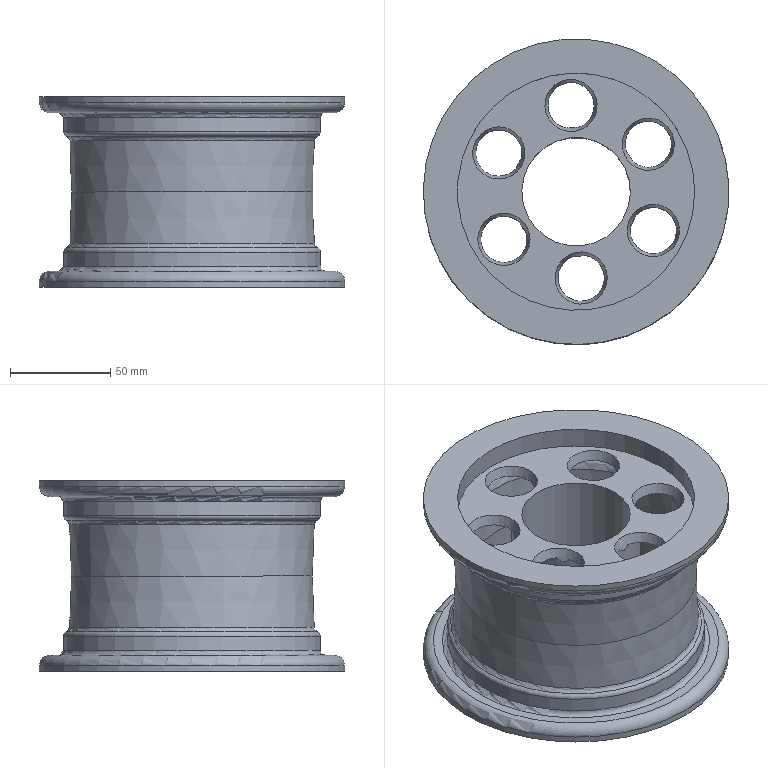Part | NX | features solid 2 | 1 solid | 44 faces | box 152.002 x 152.003 x 95.006 mm | volume 380615 mm3 | cone 16 | cylinder 10 | torus 10 | plane 8 | commonest cylinder face diameters 118 x4 128 x2 152 x2 54 x1 64 x1
STEP:
#1=CARTESIAN_POINT('',(-519.305,-904.645,30.012));
#2=VERTEX_POINT('',#1);
#3=CARTESIAN_POINT('',(-484.115,-958.102,30.014));
#4=DIRECTION('',(0.0000242,-0.00003327,-1.));
#5=DIRECTION('',(-0.5498,0.8353,-0.00004109));
#6=AXIS2_PLACEMENT_3D('',#3,#4,#5);
#7=CIRCLE('',#6,64.);
#8=EDGE_CURVE('',#2,#2,#7,.T.);
#9=ORIENTED_EDGE('',*,*,#8,.F.);
#10=EDGE_LOOP('',(#9));
#11=FACE_BOUND('',#10,.T.);
#12=CARTESIAN_POINT('',(-519.305,-904.644,37.012));
#13=VERTEX_POINT('',#12);
#14=CARTESIAN_POINT('',(-484.115,-958.102,37.014));
#15=DIRECTION('',(0.0000242,-0.00003327,-1.));
#16=DIRECTION('',(-0.5498,0.8353,-0.00004109));
#17=AXIS2_PLACEMENT_3D('',#14,#15,#16);
#18=CIRCLE('',#17,64.);
#19=EDGE_CURVE('',#13,#13,#18,.T.);
#20=ORIENTED_EDGE('',*,*,#19,.T.);
#21=EDGE_LOOP('',(#20));
#22=FACE_BOUND('',#21,.T.);
#23=CARTESIAN_POINT('',(-484.116,-958.1,73.347));
#24=DIRECTION('',(0.0000242,-0.00003327,-1.));
#25=DIRECTION('',(-0.5498,0.8353,-0.00004109));
#26=AXIS2_PLACEMENT_3D('',#23,#24,#25);
#27=CYLINDRICAL_SURFACE('',#26,64.);
#28=ADVANCED_FACE('',(#11,#22),#27,.T.);
#29=CARTESIAN_POINT('',(-518.46,-905.929,27.704));
#30=VERTEX_POINT('',#29);
#31=CARTESIAN_POINT('',(-484.115,-958.102,27.707));
#32=DIRECTION('',(0.0000242,-0.00003327,-1.));
#33=DIRECTION('',(-0.5498,0.8353,-0.00004109));
#34=AXIS2_PLACEMENT_3D('',#31,#32,#33);
#35=CIRCLE('',#34,62.462);
#36=EDGE_CURVE('',#30,#30,#35,.T.);
#37=ORIENTED_EDGE('',*,*,#36,.F.);
#38=EDGE_LOOP('',(#37));
#39=FACE_BOUND('',#38,.T.);
#40=ORIENTED_EDGE('',*,*,#8,.T.);
#41=EDGE_LOOP('',(#40));
#42=FACE_BOUND('',#41,.T.);
#43=CARTESIAN_POINT('',(-484.115,-958.102,30.014));
#44=DIRECTION('',(0.0000242,-0.00003327,-1.));
#45=DIRECTION('',(-0.5498,0.8353,-0.00004109));
#46=AXIS2_PLACEMENT_3D('',#43,#44,#45);
#47=TOROIDAL_SURFACE('',#46,61.5,2.5);
#48=ADVANCED_FACE('',(#39,#42),#47,.T.);
#49=CARTESIAN_POINT('',(-517.615,-907.212,25.488));
#50=VERTEX_POINT('',#49);
#51=CARTESIAN_POINT('',(-484.115,-958.102,25.49));
#52=DIRECTION('',(0.0000242,-0.00003327,-1.));
#53=DIRECTION('',(-0.5498,0.8353,-0.00004109));
#54=AXIS2_PLACEMENT_3D('',#51,#52,#53);
#55=CIRCLE('',#54,60.926);
#56=EDGE_CURVE('',#50,#50,#55,.T.);
#57=ORIENTED_EDGE('',*,*,#56,.F.);
#58=EDGE_LOOP('',(#57));
#59=FACE_BOUND('',#58,.T.);
#60=ORIENTED_EDGE('',*,*,#36,.T.);
#61=EDGE_LOOP('',(#60));
#62=FACE_BOUND('',#61,.T.);
#63=CARTESIAN_POINT('',(-484.115,-958.102,25.399));
#64=DIRECTION('',(0.0000242,-0.00003327,-1.));
#65=DIRECTION('',(-0.5498,0.8353,-0.00004109));
#66=AXIS2_PLACEMENT_3D('',#63,#64,#65);
#67=TOROIDAL_SURFACE('',#66,63.425,2.5);
#68=ADVANCED_FACE('',(#59,#62),#67,.F.);
#69=CARTESIAN_POINT('',(-517.105,-907.987,0.0117));
#70=VERTEX_POINT('',#69);
#71=CARTESIAN_POINT('',(-484.114,-958.103,0.01417));
#72=DIRECTION('',(0.0000242,-0.00003327,-1.));
#73=DIRECTION('',(-0.5498,0.8353,-0.00004109));
#74=AXIS2_PLACEMENT_3D('',#71,#72,#73);
#75=CIRCLE('',#74,60.);
#76=EDGE_CURVE('',#70,#70,#75,.T.);
#77=ORIENTED_EDGE('',*,*,#76,.F.);
#78=EDGE_LOOP('',(#77));
#79=FACE_BOUND('',#78,.T.);
#80=ORIENTED_EDGE('',*,*,#56,.T.);
#81=EDGE_LOOP('',(#80));
#82=FACE_BOUND('',#81,.T.);
#83=CARTESIAN_POINT('',(-484.115,-958.102,25.49));
#84=DIRECTION('',(-0.0000242,0.00003327,1.));
#85=DIRECTION('',(0.5498,-0.8353,0.00004109));
#86=AXIS2_PLACEMENT_3D('',#83,#84,#85);
#87=CONICAL_SURFACE('',#86,60.926,0.03635);
#88=ADVANCED_FACE('',(#79,#82),#87,.T.);
#89=CARTESIAN_POINT('',(-517.614,-907.214,-25.464));
#90=VERTEX_POINT('',#89);
#91=CARTESIAN_POINT('',(-484.114,-958.104,-25.462));
#92=DIRECTION('',(0.0000242,-0.00003327,-1.));
#93=DIRECTION('',(-0.5498,0.8353,-0.00004109));
#94=AXIS2_PLACEMENT_3D('',#91,#92,#93);
#95=CIRCLE('',#94,60.926);
#96=EDGE_CURVE('',#90,#90,#95,.T.);
#97=ORIENTED_EDGE('',*,*,#96,.F.);
#98=EDGE_LOOP('',(#97));
#99=FACE_BOUND('',#98,.T.);
#100=ORIENTED_EDGE('',*,*,#76,.T.);
#101=EDGE_LOOP('',(#100));
#102=FACE_BOUND('',#101,.T.);
#103=CARTESIAN_POINT('',(-484.114,-958.103,0.01417));
#104=DIRECTION('',(0.0000242,-0.00003327,-1.));
#105=DIRECTION('',(-0.5498,0.8353,-0.00004109));
#106=AXIS2_PLACEMENT_3D('',#103,#104,#105);
#107=CONICAL_SURFACE('',#106,60.,0.03635);
#108=ADVANCED_FACE('',(#99,#102),#107,.T.);
#109=CARTESIAN_POINT('',(-518.458,-905.931,-27.681));
#110=VERTEX_POINT('',#109);
#111=CARTESIAN_POINT('',(-484.114,-958.104,-27.678));
#112=DIRECTION('',(0.0000242,-0.00003327,-1.));
#113=DIRECTION('',(-0.5498,0.8353,-0.00004109));
#114=AXIS2_PLACEMENT_3D('',#111,#112,#113);
#115=CIRCLE('',#114,62.462);
#116=EDGE_CURVE('',#110,#110,#115,.T.);
#117=ORIENTED_EDGE('',*,*,#116,.F.);
#118=EDGE_LOOP('',(#117));
#119=FACE_BOUND('',#118,.T.);
#120=ORIENTED_EDGE('',*,*,#96,.T.);
#121=EDGE_LOOP('',(#120));
#122=FACE_BOUND('',#121,.T.);
#123=CARTESIAN_POINT('',(-484.114,-958.104,-25.371));
#124=DIRECTION('',(0.0000242,-0.00003327,-1.));
#125=DIRECTION('',(-0.5498,0.8353,-0.00004109));
#126=AXIS2_PLACEMENT_3D('',#123,#124,#125);
#127=TOROIDAL_SURFACE('',#126,63.425,2.5);
#128=ADVANCED_FACE('',(#119,#122),#127,.F.);
#129=CARTESIAN_POINT('',(-519.304,-904.647,-29.988));
#130=VERTEX_POINT('',#129);
#131=CARTESIAN_POINT('',(-484.114,-958.104,-29.986));
#132=DIRECTION('',(0.0000242,-0.00003327,-1.));
#133=DIRECTION('',(-0.5498,0.8353,-0.00004109));
#134=AXIS2_PLACEMENT_3D('',#131,#132,#133);
#135=CIRCLE('',#134,64.);
#136=EDGE_CURVE('',#130,#130,#135,.T.);
#137=ORIENTED_EDGE('',*,*,#136,.F.);
#138=EDGE_LOOP('',(#137));
#139=FACE_BOUND('',#138,.T.);
#140=ORIENTED_EDGE('',*,*,#116,.T.);
#141=EDGE_LOOP('',(#140));
#142=FACE_BOUND('',#141,.T.);
#143=CARTESIAN_POINT('',(-484.114,-958.104,-29.986));
#144=DIRECTION('',(0.0000242,-0.00003327,-1.));
#145=DIRECTION('',(-0.5498,0.8353,-0.00004109));
#146=AXIS2_PLACEMENT_3D('',#143,#144,#145);
#147=TOROIDAL_SURFACE('',#146,61.5,2.5);
#148=ADVANCED_FACE('',(#139,#142),#147,.T.);
#149=CARTESIAN_POINT('',(-519.303,-904.647,-36.988));
#150=VERTEX_POINT('',#149);
#151=CARTESIAN_POINT('',(-484.114,-958.104,-36.986));
#152=DIRECTION('',(0.0000242,-0.00003327,-1.));
#153=DIRECTION('',(-0.5498,0.8353,-0.00004109));
#154=AXIS2_PLACEMENT_3D('',#151,#152,#153);
#155=CIRCLE('',#154,64.);
#156=EDGE_CURVE('',#150,#150,#155,.T.);
#157=ORIENTED_EDGE('',*,*,#156,.F.);
#158=EDGE_LOOP('',(#157));
#159=FACE_BOUND('',#158,.T.);
#160=ORIENTED_EDGE('',*,*,#136,.T.);
#161=EDGE_LOOP('',(#160));
#162=FACE_BOUND('',#161,.T.);
#163=CARTESIAN_POINT('',(-484.116,-958.1,73.347));
#164=DIRECTION('',(0.0000242,-0.00003327,-1.));
#165=DIRECTION('',(-0.5498,0.8353,-0.00004109));
#166=AXIS2_PLACEMENT_3D('',#163,#164,#165);
#167=CYLINDRICAL_SURFACE('',#166,64.);
#168=ADVANCED_FACE('',(#159,#162),#167,.T.);
#169=CARTESIAN_POINT('',(-520.678,-902.559,-39.489));
#170=VERTEX_POINT('',#169);
#171=CARTESIAN_POINT('',(-484.114,-958.104,-39.486));
#172=DIRECTION('',(0.0000242,-0.00003327,-1.));
#173=DIRECTION('',(-0.5498,0.8353,-0.00004109));
#174=AXIS2_PLACEMENT_3D('',#171,#172,#173);
#175=CIRCLE('',#174,66.5);
#176=EDGE_CURVE('',#170,#170,#175,.T.);
#177=ORIENTED_EDGE('',*,*,#176,.F.);
#178=EDGE_LOOP('',(#177));
#179=FACE_BOUND('',#178,.T.);
#180=ORIENTED_EDGE('',*,*,#156,.T.);
#181=EDGE_LOOP('',(#180));
#182=FACE_BOUND('',#181,.T.);
#183=CARTESIAN_POINT('',(-484.114,-958.104,-36.986));
#184=DIRECTION('',(0.0000242,-0.00003327,-1.));
#185=DIRECTION('',(-0.5498,0.8353,-0.00004109));
#186=AXIS2_PLACEMENT_3D('',#183,#184,#185);
#187=TOROIDAL_SURFACE('',#186,66.5,2.5);
#188=ADVANCED_FACE('',(#179,#182),#187,.F.);
#189=CARTESIAN_POINT('',(-523.152,-898.8,-39.489));
#190=VERTEX_POINT('',#189);
#191=CARTESIAN_POINT('',(-484.114,-958.104,-39.486));
#192=DIRECTION('',(0.0000242,-0.00003327,-1.));
#193=DIRECTION('',(-0.5498,0.8353,-0.00004109));
#194=AXIS2_PLACEMENT_3D('',#191,#192,#193);
#195=CIRCLE('',#194,71.);
#196=EDGE_CURVE('',#190,#190,#195,.T.);
#197=ORIENTED_EDGE('',*,*,#196,.F.);
#198=EDGE_LOOP('',(#197));
#199=FACE_BOUND('',#198,.T.);
#200=ORIENTED_EDGE('',*,*,#176,.T.);
#201=EDGE_LOOP('',(#200));
#202=FACE_BOUND('',#201,.T.);
#203=CARTESIAN_POINT('',(-539.659,-994.669,-39.486));
#204=DIRECTION('',(0.0000242,-0.00003327,-1.));
#205=DIRECTION('',(-0.5498,0.8353,-0.00004109));
#206=AXIS2_PLACEMENT_3D('',#203,#204,#205);
#207=PLANE('',#206);
#208=ADVANCED_FACE('',(#199,#202),#207,.F.);
#209=CARTESIAN_POINT('',(-525.901,-894.624,-44.489));
#210=VERTEX_POINT('',#209);
#211=CARTESIAN_POINT('',(-484.113,-958.104,-44.486));
#212=DIRECTION('',(0.0000242,-0.00003327,-1.));
#213=DIRECTION('',(-0.5498,0.8353,-0.00004109));
#214=AXIS2_PLACEMENT_3D('',#211,#212,#213);
#215=CIRCLE('',#214,76.);
#216=EDGE_CURVE('',#210,#210,#215,.T.);
#217=ORIENTED_EDGE('',*,*,#216,.F.);
#218=EDGE_LOOP('',(#217));
#219=FACE_BOUND('',#218,.T.);
#220=ORIENTED_EDGE('',*,*,#196,.T.);
#221=EDGE_LOOP('',(#220));
#222=FACE_BOUND('',#221,.T.);
#223=CARTESIAN_POINT('',(-484.113,-958.104,-44.486));
#224=DIRECTION('',(0.0000242,-0.00003327,-1.));
#225=DIRECTION('',(-0.5498,0.8353,-0.00004109));
#226=AXIS2_PLACEMENT_3D('',#223,#224,#225);
#227=TOROIDAL_SURFACE('',#226,71.,5.);
#228=ADVANCED_FACE('',(#219,#222),#227,.T.);
#229=CARTESIAN_POINT('',(-525.901,-894.624,-47.489));
#230=VERTEX_POINT('',#229);
#231=CARTESIAN_POINT('',(-484.113,-958.105,-47.486));
#232=DIRECTION('',(0.0000242,-0.00003327,-1.));
#233=DIRECTION('',(-0.5498,0.8353,-0.00004109));
#234=AXIS2_PLACEMENT_3D('',#231,#232,#233);
#235=CIRCLE('',#234,76.);
#236=EDGE_CURVE('',#230,#230,#235,.T.);
#237=ORIENTED_EDGE('',*,*,#236,.F.);
#238=EDGE_LOOP('',(#237));
#239=FACE_BOUND('',#238,.T.);
#240=ORIENTED_EDGE('',*,*,#216,.T.);
#241=EDGE_LOOP('',(#240));
#242=FACE_BOUND('',#241,.T.);
#243=CARTESIAN_POINT('',(-484.116,-958.1,73.347));
#244=DIRECTION('',(0.0000242,-0.00003327,-1.));
#245=DIRECTION('',(-0.5498,0.8353,-0.00004109));
#246=AXIS2_PLACEMENT_3D('',#243,#244,#245);
#247=CYLINDRICAL_SURFACE('',#246,76.);
#248=ADVANCED_FACE('',(#239,#242),#247,.T.);
#249=CARTESIAN_POINT('',(-516.554,-908.824,-47.488));
#250=VERTEX_POINT('',#249);
#251=CARTESIAN_POINT('',(-484.113,-958.105,-47.486));
#252=DIRECTION('',(0.0000242,-0.00003327,-1.));
#253=DIRECTION('',(-0.5498,0.8353,-0.00004109));
#254=AXIS2_PLACEMENT_3D('',#251,#252,#253);
#255=CIRCLE('',#254,59.);
#256=EDGE_CURVE('',#250,#250,#255,.T.);
#257=ORIENTED_EDGE('',*,*,#256,.F.);
#258=EDGE_LOOP('',(#257));
#259=FACE_BOUND('',#258,.T.);
#260=ORIENTED_EDGE('',*,*,#236,.T.);
#261=EDGE_LOOP('',(#260));
#262=FACE_BOUND('',#261,.T.);
#263=CARTESIAN_POINT('',(-547.594,-999.892,-47.486));
#264=DIRECTION('',(-0.0000242,0.00003327,1.));
#265=DIRECTION('',(0.5498,-0.8353,0.00004109));
#266=AXIS2_PLACEMENT_3D('',#263,#264,#265);
#267=PLANE('',#266);
#268=ADVANCED_FACE('',(#259,#262),#267,.F.);
#269=CARTESIAN_POINT('',(-516.554,-908.823,-37.488));
#270=VERTEX_POINT('',#269);
#271=CARTESIAN_POINT('',(-484.114,-958.104,-37.486));
#272=DIRECTION('',(0.0000242,-0.00003327,-1.));
#273=DIRECTION('',(-0.5498,0.8353,-0.00004109));
#274=AXIS2_PLACEMENT_3D('',#271,#272,#273);
#275=CIRCLE('',#274,59.);
#276=EDGE_CURVE('',#270,#270,#275,.T.);
#277=ORIENTED_EDGE('',*,*,#276,.F.);
#278=EDGE_LOOP('',(#277));
#279=FACE_BOUND('',#278,.T.);
#280=ORIENTED_EDGE('',*,*,#256,.T.);
#281=EDGE_LOOP('',(#280));
#282=FACE_BOUND('',#281,.T.);
#283=CARTESIAN_POINT('',(-484.116,-958.1,73.347));
#284=DIRECTION('',(0.0000242,-0.00003327,-1.));
#285=DIRECTION('',(-0.5498,0.8353,-0.00004109));
#286=AXIS2_PLACEMENT_3D('',#283,#284,#285);
#287=CYLINDRICAL_SURFACE('',#286,59.);
#288=ADVANCED_FACE('',(#279,#282),#287,.F.);
#289=CARTESIAN_POINT('',(-468.619,-1000.269,-37.484));
#290=VERTEX_POINT('',#289);
#291=CARTESIAN_POINT('',(-481.596,-1001.03,-37.484));
#292=DIRECTION('',(-0.0000242,0.00003327,1.));
#293=DIRECTION('',(0.9983,0.05854,0.00002221));
#294=AXIS2_PLACEMENT_3D('',#291,#292,#293);
#295=CIRCLE('',#294,13.);
#296=EDGE_CURVE('',#290,#290,#295,.T.);
#297=ORIENTED_EDGE('',*,*,#296,.T.);
#298=EDGE_LOOP('',(#297));
#299=FACE_BOUND('',#298,.T.);
#300=CARTESIAN_POINT('',(-439.85,-965.768,-37.485));
#301=VERTEX_POINT('',#300);
#302=CARTESIAN_POINT('',(-445.68,-977.387,-37.484));
#303=DIRECTION('',(-0.0000242,0.00003327,1.));
#304=DIRECTION('',(0.4484,0.8938,-0.00001889));
#305=AXIS2_PLACEMENT_3D('',#302,#303,#304);
#306=CIRCLE('',#305,13.);
#307=EDGE_CURVE('',#301,#301,#306,.T.);
#308=ORIENTED_EDGE('',*,*,#307,.T.);
#309=EDGE_LOOP('',(#308));
#310=FACE_BOUND('',#309,.T.);
#311=CARTESIAN_POINT('',(-455.345,-923.603,-37.486));
#312=VERTEX_POINT('',#311);
#313=CARTESIAN_POINT('',(-448.197,-934.461,-37.486));
#314=DIRECTION('',(-0.0000242,0.00003327,1.));
#315=DIRECTION('',(-0.5498,0.8353,-0.00004109));
#316=AXIS2_PLACEMENT_3D('',#313,#314,#315);
#317=CIRCLE('',#316,13.);
#318=EDGE_CURVE('',#312,#312,#317,.T.);
#319=ORIENTED_EDGE('',*,*,#318,.T.);
#320=EDGE_LOOP('',(#319));
#321=FACE_BOUND('',#320,.T.);
#322=CARTESIAN_POINT('',(-499.609,-915.939,-37.488));
#323=VERTEX_POINT('',#322);
#324=CARTESIAN_POINT('',(-486.631,-915.178,-37.487));
#325=DIRECTION('',(-0.0000242,0.00003327,1.));
#326=DIRECTION('',(-0.9983,-0.05854,-0.00002221));
#327=AXIS2_PLACEMENT_3D('',#324,#325,#326);
#328=CIRCLE('',#327,13.);
#329=EDGE_CURVE('',#323,#323,#328,.T.);
#330=ORIENTED_EDGE('',*,*,#329,.T.);
#331=EDGE_LOOP('',(#330));
#332=FACE_BOUND('',#331,.T.);
#333=CARTESIAN_POINT('',(-528.377,-950.441,-37.487));
#334=VERTEX_POINT('',#333);
#335=CARTESIAN_POINT('',(-522.547,-938.821,-37.487));
#336=DIRECTION('',(-0.0000242,0.00003327,1.));
#337=DIRECTION('',(-0.4484,-0.8938,0.00001889));
#338=AXIS2_PLACEMENT_3D('',#335,#336,#337);
#339=CIRCLE('',#338,13.);
#340=EDGE_CURVE('',#334,#334,#339,.T.);
#341=ORIENTED_EDGE('',*,*,#340,.T.);
#342=EDGE_LOOP('',(#341));
#343=FACE_BOUND('',#342,.T.);
#344=CARTESIAN_POINT('',(-512.882,-992.606,-37.485));
#345=VERTEX_POINT('',#344);
#346=CARTESIAN_POINT('',(-520.03,-981.747,-37.486));
#347=DIRECTION('',(-0.0000242,0.00003327,1.));
#348=DIRECTION('',(0.5498,-0.8353,0.00004109));
#349=AXIS2_PLACEMENT_3D('',#346,#347,#348);
#350=CIRCLE('',#349,13.);
#351=EDGE_CURVE('',#345,#345,#350,.T.);
#352=ORIENTED_EDGE('',*,*,#351,.T.);
#353=EDGE_LOOP('',(#352));
#354=FACE_BOUND('',#353,.T.);
#355=CARTESIAN_POINT('',(-498.959,-935.552,-37.487));
#356=VERTEX_POINT('',#355);
#357=CARTESIAN_POINT('',(-484.114,-958.104,-37.486));
#358=DIRECTION('',(0.0000242,-0.00003327,-1.));
#359=DIRECTION('',(-0.5498,0.8353,-0.00004109));
#360=AXIS2_PLACEMENT_3D('',#357,#358,#359);
#361=CIRCLE('',#360,27.);
#362=EDGE_CURVE('',#356,#356,#361,.T.);
#363=ORIENTED_EDGE('',*,*,#362,.F.);
#364=EDGE_LOOP('',(#363));
#365=FACE_BOUND('',#364,.T.);
#366=ORIENTED_EDGE('',*,*,#276,.T.);
#367=EDGE_LOOP('',(#366));
#368=FACE_BOUND('',#367,.T.);
#369=CARTESIAN_POINT('',(-533.394,-990.545,-37.486));
#370=DIRECTION('',(-0.0000242,0.00003327,1.));
#371=DIRECTION('',(0.5498,-0.8353,0.00004109));
#372=AXIS2_PLACEMENT_3D('',#369,#370,#371);
#373=PLANE('',#372);
#374=ADVANCED_FACE('',(#299,#310,#321,#332,#343,#354,#365,#368),#373,.F.);
#375=CARTESIAN_POINT('',(-498.961,-935.549,37.513));
#376=VERTEX_POINT('',#375);
#377=CARTESIAN_POINT('',(-484.115,-958.102,37.514));
#378=DIRECTION('',(0.0000242,-0.00003327,-1.));
#379=DIRECTION('',(-0.5498,0.8353,-0.00004109));
#380=AXIS2_PLACEMENT_3D('',#377,#378,#379);
#381=CIRCLE('',#380,27.);
#382=EDGE_CURVE('',#376,#376,#381,.T.);
#383=ORIENTED_EDGE('',*,*,#382,.F.);
#384=EDGE_LOOP('',(#383));
#385=FACE_BOUND('',#384,.T.);
#386=ORIENTED_EDGE('',*,*,#362,.T.);
#387=EDGE_LOOP('',(#386));
#388=FACE_BOUND('',#387,.T.);
#389=CARTESIAN_POINT('',(-484.116,-958.1,73.347));
#390=DIRECTION('',(0.0000242,-0.00003327,-1.));
#391=DIRECTION('',(-0.5498,0.8353,-0.00004109));
#392=AXIS2_PLACEMENT_3D('',#389,#390,#391);
#393=CYLINDRICAL_SURFACE('',#392,27.);
#394=ADVANCED_FACE('',(#385,#388),#393,.F.);
#395=CARTESIAN_POINT('',(-468.62,-1000.267,37.516));
#396=VERTEX_POINT('',#395);
#397=CARTESIAN_POINT('',(-481.598,-1001.028,37.516));
#398=DIRECTION('',(-0.0000242,0.00003327,1.));
#399=DIRECTION('',(0.9983,0.05854,0.00002221));
#400=AXIS2_PLACEMENT_3D('',#397,#398,#399);
#401=CIRCLE('',#400,13.);
#402=EDGE_CURVE('',#396,#396,#401,.T.);
#403=ORIENTED_EDGE('',*,*,#402,.F.);
#404=EDGE_LOOP('',(#403));
#405=FACE_BOUND('',#404,.T.);
#406=CARTESIAN_POINT('',(-439.852,-965.765,37.515));
#407=VERTEX_POINT('',#406);
#408=CARTESIAN_POINT('',(-445.682,-977.385,37.516));
#409=DIRECTION('',(-0.0000242,0.00003327,1.));
#410=DIRECTION('',(0.4484,0.8938,-0.00001889));
#411=AXIS2_PLACEMENT_3D('',#408,#409,#410);
#412=CIRCLE('',#411,13.);
#413=EDGE_CURVE('',#407,#407,#412,.T.);
#414=ORIENTED_EDGE('',*,*,#413,.F.);
#415=EDGE_LOOP('',(#414));
#416=FACE_BOUND('',#415,.T.);
#417=CARTESIAN_POINT('',(-455.347,-923.6,37.514));
#418=VERTEX_POINT('',#417);
#419=CARTESIAN_POINT('',(-448.199,-934.459,37.514));
#420=DIRECTION('',(-0.0000242,0.00003327,1.));
#421=DIRECTION('',(-0.5498,0.8353,-0.00004109));
#422=AXIS2_PLACEMENT_3D('',#419,#420,#421);
#423=CIRCLE('',#422,13.);
#424=EDGE_CURVE('',#418,#418,#423,.T.);
#425=ORIENTED_EDGE('',*,*,#424,.F.);
#426=EDGE_LOOP('',(#425));
#427=FACE_BOUND('',#426,.T.);
#428=CARTESIAN_POINT('',(-499.61,-915.936,37.512));
#429=VERTEX_POINT('',#428);
#430=CARTESIAN_POINT('',(-486.633,-915.175,37.513));
#431=DIRECTION('',(-0.0000242,0.00003327,1.));
#432=DIRECTION('',(-0.9983,-0.05854,-0.00002221));
#433=AXIS2_PLACEMENT_3D('',#430,#431,#432);
#434=CIRCLE('',#433,13.);
#435=EDGE_CURVE('',#429,#429,#434,.T.);
#436=ORIENTED_EDGE('',*,*,#435,.F.);
#437=EDGE_LOOP('',(#436));
#438=FACE_BOUND('',#437,.T.);
#439=CARTESIAN_POINT('',(-528.379,-950.438,37.513));
#440=VERTEX_POINT('',#439);
#441=CARTESIAN_POINT('',(-522.549,-938.819,37.513));
#442=DIRECTION('',(-0.0000242,0.00003327,1.));
#443=DIRECTION('',(-0.4484,-0.8938,0.00001889));
#444=AXIS2_PLACEMENT_3D('',#441,#442,#443);
#445=CIRCLE('',#444,13.);
#446=EDGE_CURVE('',#440,#440,#445,.T.);
#447=ORIENTED_EDGE('',*,*,#446,.F.);
#448=EDGE_LOOP('',(#447));
#449=FACE_BOUND('',#448,.T.);
#450=CARTESIAN_POINT('',(-512.884,-992.603,37.515));
#451=VERTEX_POINT('',#450);
#452=CARTESIAN_POINT('',(-520.032,-981.745,37.514));
#453=DIRECTION('',(-0.0000242,0.00003327,1.));
#454=DIRECTION('',(0.5498,-0.8353,0.00004109));
#455=AXIS2_PLACEMENT_3D('',#452,#453,#454);
#456=CIRCLE('',#455,13.);
#457=EDGE_CURVE('',#451,#451,#456,.T.);
#458=ORIENTED_EDGE('',*,*,#457,.F.);
#459=EDGE_LOOP('',(#458));
#460=FACE_BOUND('',#459,.T.);
#461=CARTESIAN_POINT('',(-516.556,-908.821,37.512));
#462=VERTEX_POINT('',#461);
#463=CARTESIAN_POINT('',(-484.115,-958.102,37.514));
#464=DIRECTION('',(0.0000242,-0.00003327,-1.));
#465=DIRECTION('',(-0.5498,0.8353,-0.00004109));
#466=AXIS2_PLACEMENT_3D('',#463,#464,#465);
#467=CIRCLE('',#466,59.);
#468=EDGE_CURVE('',#462,#462,#467,.T.);
#469=ORIENTED_EDGE('',*,*,#468,.F.);
#470=EDGE_LOOP('',(#469));
#471=FACE_BOUND('',#470,.T.);
#472=ORIENTED_EDGE('',*,*,#382,.T.);
#473=EDGE_LOOP('',(#472));
#474=FACE_BOUND('',#473,.T.);
#475=CARTESIAN_POINT('',(-506.668,-972.947,37.514));
#476=DIRECTION('',(0.0000242,-0.00003327,-1.));
#477=DIRECTION('',(-0.5498,0.8353,-0.00004109));
#478=AXIS2_PLACEMENT_3D('',#475,#476,#477);
#479=PLANE('',#478);
#480=ADVANCED_FACE('',(#405,#416,#427,#438,#449,#460,#471,#474),#479,.F.);
#481=CARTESIAN_POINT('',(-516.556,-908.82,47.512));
#482=VERTEX_POINT('',#481);
#483=CARTESIAN_POINT('',(-484.116,-958.101,47.514));
#484=DIRECTION('',(0.0000242,-0.00003327,-1.));
#485=DIRECTION('',(-0.5498,0.8353,-0.00004109));
#486=AXIS2_PLACEMENT_3D('',#483,#484,#485);
#487=CIRCLE('',#486,59.);
#488=EDGE_CURVE('',#482,#482,#487,.T.);
#489=ORIENTED_EDGE('',*,*,#488,.F.);
#490=EDGE_LOOP('',(#489));
#491=FACE_BOUND('',#490,.T.);
#492=ORIENTED_EDGE('',*,*,#468,.T.);
#493=EDGE_LOOP('',(#492));
#494=FACE_BOUND('',#493,.T.);
#495=CARTESIAN_POINT('',(-484.116,-958.1,73.347));
#496=DIRECTION('',(0.0000242,-0.00003327,-1.));
#497=DIRECTION('',(-0.5498,0.8353,-0.00004109));
#498=AXIS2_PLACEMENT_3D('',#495,#496,#497);
#499=CYLINDRICAL_SURFACE('',#498,59.);
#500=ADVANCED_FACE('',(#491,#494),#499,.F.);
#501=CARTESIAN_POINT('',(-525.904,-894.621,47.511));
#502=VERTEX_POINT('',#501);
#503=CARTESIAN_POINT('',(-484.116,-958.101,47.514));
#504=DIRECTION('',(0.0000242,-0.00003327,-1.));
#505=DIRECTION('',(-0.5498,0.8353,-0.00004109));
#506=AXIS2_PLACEMENT_3D('',#503,#504,#505);
#507=CIRCLE('',#506,76.);
#508=EDGE_CURVE('',#502,#502,#507,.T.);
#509=ORIENTED_EDGE('',*,*,#508,.F.);
#510=EDGE_LOOP('',(#509));
#511=FACE_BOUND('',#510,.T.);
#512=ORIENTED_EDGE('',*,*,#488,.T.);
#513=EDGE_LOOP('',(#512));
#514=FACE_BOUND('',#513,.T.);
#515=CARTESIAN_POINT('',(-533.397,-990.542,47.514));
#516=DIRECTION('',(0.0000242,-0.00003327,-1.));
#517=DIRECTION('',(-0.5498,0.8353,-0.00004109));
#518=AXIS2_PLACEMENT_3D('',#515,#516,#517);
#519=PLANE('',#518);
#520=ADVANCED_FACE('',(#511,#514),#519,.F.);
#521=CARTESIAN_POINT('',(-525.903,-894.621,44.511));
#522=VERTEX_POINT('',#521);
#523=CARTESIAN_POINT('',(-484.116,-958.101,44.514));
#524=DIRECTION('',(0.0000242,-0.00003327,-1.));
#525=DIRECTION('',(-0.5498,0.8353,-0.00004109));
#526=AXIS2_PLACEMENT_3D('',#523,#524,#525);
#527=CIRCLE('',#526,76.);
#528=EDGE_CURVE('',#522,#522,#527,.T.);
#529=ORIENTED_EDGE('',*,*,#528,.F.);
#530=EDGE_LOOP('',(#529));
#531=FACE_BOUND('',#530,.T.);
#532=ORIENTED_EDGE('',*,*,#508,.T.);
#533=EDGE_LOOP('',(#532));
#534=FACE_BOUND('',#533,.T.);
#535=CARTESIAN_POINT('',(-484.116,-958.1,73.347));
#536=DIRECTION('',(0.0000242,-0.00003327,-1.));
#537=DIRECTION('',(-0.5498,0.8353,-0.00004109));
#538=AXIS2_PLACEMENT_3D('',#535,#536,#537);
#539=CYLINDRICAL_SURFACE('',#538,76.);
#540=ADVANCED_FACE('',(#531,#534),#539,.T.);
#541=CARTESIAN_POINT('',(-523.154,-898.797,39.511));
#542=VERTEX_POINT('',#541);
#543=CARTESIAN_POINT('',(-484.115,-958.102,39.514));
#544=DIRECTION('',(0.0000242,-0.00003327,-1.));
#545=DIRECTION('',(-0.5498,0.8353,-0.00004109));
#546=AXIS2_PLACEMENT_3D('',#543,#544,#545);
#547=CIRCLE('',#546,71.);
#548=EDGE_CURVE('',#542,#542,#547,.T.);
#549=ORIENTED_EDGE('',*,*,#548,.F.);
#550=EDGE_LOOP('',(#549));
#551=FACE_BOUND('',#550,.T.);
#552=ORIENTED_EDGE('',*,*,#528,.T.);
#553=EDGE_LOOP('',(#552));
#554=FACE_BOUND('',#553,.T.);
#555=CARTESIAN_POINT('',(-484.116,-958.101,44.514));
#556=DIRECTION('',(0.0000242,-0.00003327,-1.));
#557=DIRECTION('',(-0.5498,0.8353,-0.00004109));
#558=AXIS2_PLACEMENT_3D('',#555,#556,#557);
#559=TOROIDAL_SURFACE('',#558,71.,5.);
#560=ADVANCED_FACE('',(#551,#554),#559,.T.);
#561=CARTESIAN_POINT('',(-520.68,-902.556,39.511));
#562=VERTEX_POINT('',#561);
#563=CARTESIAN_POINT('',(-484.115,-958.102,39.514));
#564=DIRECTION('',(0.0000242,-0.00003327,-1.));
#565=DIRECTION('',(-0.5498,0.8353,-0.00004109));
#566=AXIS2_PLACEMENT_3D('',#563,#564,#565);
#567=CIRCLE('',#566,66.5);
#568=EDGE_CURVE('',#562,#562,#567,.T.);
#569=ORIENTED_EDGE('',*,*,#568,.F.);
#570=EDGE_LOOP('',(#569));
#571=FACE_BOUND('',#570,.T.);
#572=ORIENTED_EDGE('',*,*,#548,.T.);
#573=EDGE_LOOP('',(#572));
#574=FACE_BOUND('',#573,.T.);
#575=CARTESIAN_POINT('',(-543.42,-997.14,39.514));
#576=DIRECTION('',(-0.0000242,0.00003327,1.));
#577=DIRECTION('',(0.5498,-0.8353,0.00004109));
#578=AXIS2_PLACEMENT_3D('',#575,#576,#577);
#579=PLANE('',#578);
#580=ADVANCED_FACE('',(#571,#574),#579,.F.);
#581=ORIENTED_EDGE('',*,*,#19,.F.);
#582=EDGE_LOOP('',(#581));
#583=FACE_BOUND('',#582,.T.);
#584=ORIENTED_EDGE('',*,*,#568,.T.);
#585=EDGE_LOOP('',(#584));
#586=FACE_BOUND('',#585,.T.);
#587=CARTESIAN_POINT('',(-484.115,-958.102,37.014));
#588=DIRECTION('',(0.0000242,-0.00003327,-1.));
#589=DIRECTION('',(-0.5498,0.8353,-0.00004109));
#590=AXIS2_PLACEMENT_3D('',#587,#588,#589);
#591=TOROIDAL_SURFACE('',#590,66.5,2.5);
#592=ADVANCED_FACE('',(#583,#586),#591,.F.);
#593=CARTESIAN_POINT('',(-509.102,-978.093,-32.486));
#594=VERTEX_POINT('',#593);
#595=CARTESIAN_POINT('',(-512.354,-973.154,-32.486));
#596=VERTEX_POINT('',#595);
#597=CARTESIAN_POINT('',(-509.102,-978.093,-32.486));
#598=CARTESIAN_POINT('',(-509.344,-977.792,-32.035));
#599=CARTESIAN_POINT('',(-509.851,-977.14,-31.194));
#600=CARTESIAN_POINT('',(-510.854,-975.714,-30.48));
#601=CARTESIAN_POINT('',(-511.769,-974.227,-31.185));
#602=CARTESIAN_POINT('',(-512.172,-973.496,-32.034));
#603=CARTESIAN_POINT('',(-512.354,-973.154,-32.486));
#604=B_SPLINE_CURVE_WITH_KNOTS('',3,(#597,#598,#599,#600,#601,#602,#603),.UNSPECIFIED.,.F.,.F.,(4,1,1,1,4),(0.000000261,0.001766,0.003532,0.005299,0.007065),.UNSPECIFIED.);
#605=EDGE_CURVE('',#594,#596,#604,.T.);
#606=ORIENTED_EDGE('',*,*,#605,.T.);
#607=CARTESIAN_POINT('',(-520.03,-981.747,-32.486));
#608=DIRECTION('',(-0.0000242,0.00003327,1.));
#609=DIRECTION('',(0.5498,-0.8353,0.00004109));
#610=AXIS2_PLACEMENT_3D('',#607,#608,#609);
#611=CIRCLE('',#610,11.523);
#612=EDGE_CURVE('',#596,#594,#611,.T.);
#613=ORIENTED_EDGE('',*,*,#612,.T.);
#614=EDGE_LOOP('',(#606,#613));
#615=FACE_BOUND('',#614,.T.);
#616=ORIENTED_EDGE('',*,*,#351,.F.);
#617=EDGE_LOOP('',(#616));
#618=FACE_BOUND('',#617,.T.);
#619=CARTESIAN_POINT('',(-520.031,-981.747,-15.486));
#620=DIRECTION('',(0.0000242,-0.00003327,-1.));
#621=DIRECTION('',(-0.5498,0.8353,-0.00004109));
#622=AXIS2_PLACEMENT_3D('',#619,#620,#621);
#623=CONICAL_SURFACE('',#622,6.5,0.2873);
#624=ADVANCED_FACE('',(#615,#618),#623,.F.);
#625=CARTESIAN_POINT('',(-509.104,-978.091,32.514));
#626=VERTEX_POINT('',#625);
#627=CARTESIAN_POINT('',(-512.355,-973.152,32.514));
#628=VERTEX_POINT('',#627);
#629=CARTESIAN_POINT('',(-520.032,-981.745,32.514));
#630=DIRECTION('',(0.0000242,-0.00003327,-1.));
#631=DIRECTION('',(-0.5498,0.8353,-0.00004109));
#632=AXIS2_PLACEMENT_3D('',#629,#630,#631);
#633=CIRCLE('',#632,11.523);
#634=EDGE_CURVE('',#626,#628,#633,.T.);
#635=ORIENTED_EDGE('',*,*,#634,.T.);
#636=CARTESIAN_POINT('',(-512.355,-973.152,32.514));
#637=CARTESIAN_POINT('',(-512.174,-973.493,32.063));
#638=CARTESIAN_POINT('',(-511.776,-974.216,31.222));
#639=CARTESIAN_POINT('',(-510.862,-975.701,30.508));
#640=CARTESIAN_POINT('',(-509.858,-977.13,31.213));
#641=CARTESIAN_POINT('',(-509.346,-977.789,32.062));
#642=CARTESIAN_POINT('',(-509.104,-978.091,32.514));
#643=B_SPLINE_CURVE_WITH_KNOTS('',3,(#636,#637,#638,#639,#640,#641,#642),.UNSPECIFIED.,.F.,.F.,(4,1,1,1,4),(0.000000261,0.001766,0.003532,0.005299,0.007065),.UNSPECIFIED.);
#644=EDGE_CURVE('',#628,#626,#643,.T.);
#645=ORIENTED_EDGE('',*,*,#644,.T.);
#646=EDGE_LOOP('',(#635,#645));
#647=FACE_BOUND('',#646,.T.);
#648=ORIENTED_EDGE('',*,*,#457,.T.);
#649=EDGE_LOOP('',(#648));
#650=FACE_BOUND('',#649,.T.);
#651=CARTESIAN_POINT('',(-520.032,-981.745,37.514));
#652=DIRECTION('',(-0.0000242,0.00003327,1.));
#653=DIRECTION('',(0.5498,-0.8353,0.00004109));
#654=AXIS2_PLACEMENT_3D('',#651,#652,#653);
#655=CONICAL_SURFACE('',#654,13.,0.2873);
#656=ADVANCED_FACE('',(#647,#650),#655,.F.);
#657=CARTESIAN_POINT('',(-516.554,-908.823,-31.429));
#658=VERTEX_POINT('',#657);
#659=CARTESIAN_POINT('',(-484.114,-958.104,-31.427));
#660=DIRECTION('',(0.0000242,-0.00003327,-1.));
#661=DIRECTION('',(-0.5498,0.8353,-0.00004109));
#662=AXIS2_PLACEMENT_3D('',#659,#660,#661);
#663=CIRCLE('',#662,59.);
#664=EDGE_CURVE('',#658,#658,#663,.T.);
#665=ORIENTED_EDGE('',*,*,#664,.T.);
#666=EDGE_LOOP('',(#665));
#667=FACE_BOUND('',#666,.T.);
#668=CARTESIAN_POINT('',(-514.866,-911.387,-25.646));
#669=VERTEX_POINT('',#668);
#670=CARTESIAN_POINT('',(-484.114,-958.104,-25.644));
#671=DIRECTION('',(0.0000242,-0.00003327,-1.));
#672=DIRECTION('',(-0.5498,0.8353,-0.00004109));
#673=AXIS2_PLACEMENT_3D('',#670,#671,#672);
#674=CIRCLE('',#673,55.93);
#675=EDGE_CURVE('',#669,#669,#674,.T.);
#676=ORIENTED_EDGE('',*,*,#675,.F.);
#677=EDGE_LOOP('',(#676));
#678=FACE_BOUND('',#677,.T.);
#679=CARTESIAN_POINT('',(-484.114,-958.104,-25.371));
#680=DIRECTION('',(0.0000242,-0.00003327,-1.));
#681=DIRECTION('',(-0.5498,0.8353,-0.00004109));
#682=AXIS2_PLACEMENT_3D('',#679,#680,#681);
#683=TOROIDAL_SURFACE('',#682,63.425,7.5);
#684=ADVANCED_FACE('',(#667,#678),#683,.T.);
#685=ORIENTED_EDGE('',*,*,#675,.T.);
#686=EDGE_LOOP('',(#685));
#687=FACE_BOUND('',#686,.T.);
#688=CARTESIAN_POINT('',(-514.354,-912.166,0.01191));
#689=VERTEX_POINT('',#688);
#690=CARTESIAN_POINT('',(-484.114,-958.103,0.01417));
#691=DIRECTION('',(0.0000242,-0.00003327,-1.));
#692=DIRECTION('',(-0.5498,0.8353,-0.00004109));
#693=AXIS2_PLACEMENT_3D('',#690,#691,#692);
#694=CIRCLE('',#693,54.997);
#695=EDGE_CURVE('',#689,#689,#694,.T.);
#696=ORIENTED_EDGE('',*,*,#695,.F.);
#697=EDGE_LOOP('',(#696));
#698=FACE_BOUND('',#697,.T.);
#699=CARTESIAN_POINT('',(-484.114,-958.103,0.01417));
#700=DIRECTION('',(0.0000242,-0.00003327,-1.));
#701=DIRECTION('',(-0.5498,0.8353,-0.00004109));
#702=AXIS2_PLACEMENT_3D('',#699,#700,#701);
#703=CONICAL_SURFACE('',#702,54.997,0.03635);
#704=ADVANCED_FACE('',(#687,#698),#703,.F.);
#705=ORIENTED_EDGE('',*,*,#695,.T.);
#706=EDGE_LOOP('',(#705));
#707=FACE_BOUND('',#706,.T.);
#708=CARTESIAN_POINT('',(-514.868,-911.386,25.67));
#709=VERTEX_POINT('',#708);
#710=CARTESIAN_POINT('',(-484.115,-958.102,25.672));
#711=DIRECTION('',(0.0000242,-0.00003327,-1.));
#712=DIRECTION('',(-0.5498,0.8353,-0.00004109));
#713=AXIS2_PLACEMENT_3D('',#710,#711,#712);
#714=CIRCLE('',#713,55.93);
#715=EDGE_CURVE('',#709,#709,#714,.T.);
#716=ORIENTED_EDGE('',*,*,#715,.F.);
#717=EDGE_LOOP('',(#716));
#718=FACE_BOUND('',#717,.T.);
#719=CARTESIAN_POINT('',(-484.115,-958.102,25.672));
#720=DIRECTION('',(-0.0000242,0.00003327,1.));
#721=DIRECTION('',(0.5498,-0.8353,0.00004109));
#722=AXIS2_PLACEMENT_3D('',#719,#720,#721);
#723=CONICAL_SURFACE('',#722,55.93,0.03635);
#724=ADVANCED_FACE('',(#707,#718),#723,.F.);
#725=ORIENTED_EDGE('',*,*,#715,.T.);
#726=EDGE_LOOP('',(#725));
#727=FACE_BOUND('',#726,.T.);
#728=CARTESIAN_POINT('',(-516.556,-908.821,31.453));
#729=VERTEX_POINT('',#728);
#730=CARTESIAN_POINT('',(-484.115,-958.102,31.455));
#731=DIRECTION('',(0.0000242,-0.00003327,-1.));
#732=DIRECTION('',(-0.5498,0.8353,-0.00004109));
#733=AXIS2_PLACEMENT_3D('',#730,#731,#732);
#734=CIRCLE('',#733,59.);
#735=EDGE_CURVE('',#729,#729,#734,.T.);
#736=ORIENTED_EDGE('',*,*,#735,.F.);
#737=EDGE_LOOP('',(#736));
#738=FACE_BOUND('',#737,.T.);
#739=CARTESIAN_POINT('',(-484.115,-958.102,25.399));
#740=DIRECTION('',(0.0000242,-0.00003327,-1.));
#741=DIRECTION('',(-0.5498,0.8353,-0.00004109));
#742=AXIS2_PLACEMENT_3D('',#739,#740,#741);
#743=TOROIDAL_SURFACE('',#742,63.425,7.5);
#744=ADVANCED_FACE('',(#727,#738),#743,.T.);
#745=ORIENTED_EDGE('',*,*,#735,.T.);
#746=EDGE_LOOP('',(#745));
#747=FACE_BOUND('',#746,.T.);
#748=CARTESIAN_POINT('',(-516.556,-908.821,32.512));
#749=VERTEX_POINT('',#748);
#750=CARTESIAN_POINT('',(-484.115,-958.102,32.514));
#751=DIRECTION('',(0.0000242,-0.00003327,-1.));
#752=DIRECTION('',(-0.5498,0.8353,-0.00004109));
#753=AXIS2_PLACEMENT_3D('',#750,#751,#752);
#754=CIRCLE('',#753,59.);
#755=EDGE_CURVE('',#749,#749,#754,.T.);
#756=ORIENTED_EDGE('',*,*,#755,.F.);
#757=EDGE_LOOP('',(#756));
#758=FACE_BOUND('',#757,.T.);
#759=CARTESIAN_POINT('',(-484.116,-958.1,73.347));
#760=DIRECTION('',(0.0000242,-0.00003327,-1.));
#761=DIRECTION('',(-0.5498,0.8353,-0.00004109));
#762=AXIS2_PLACEMENT_3D('',#759,#760,#761);
#763=CYLINDRICAL_SURFACE('',#762,59.);
#764=ADVANCED_FACE('',(#747,#758),#763,.F.);
#765=CARTESIAN_POINT('',(-479.298,-989.737,32.515));
#766=VERTEX_POINT('',#765);
#767=CARTESIAN_POINT('',(-485.202,-990.083,32.515));
#768=VERTEX_POINT('',#767);
#769=CARTESIAN_POINT('',(-481.598,-1001.028,32.516));
#770=DIRECTION('',(0.0000242,-0.00003327,-1.));
#771=DIRECTION('',(-0.5498,0.8353,-0.00004109));
#772=AXIS2_PLACEMENT_3D('',#769,#770,#771);
#773=CIRCLE('',#772,11.523);
#774=EDGE_CURVE('',#766,#768,#773,.T.);
#775=ORIENTED_EDGE('',*,*,#774,.F.);
#776=CARTESIAN_POINT('',(-456.962,-975.034,32.515));
#777=VERTEX_POINT('',#776);
#778=CARTESIAN_POINT('',(-484.115,-958.102,32.514));
#779=DIRECTION('',(0.0000242,-0.00003327,-1.));
#780=DIRECTION('',(-0.5498,0.8353,-0.00004109));
#781=AXIS2_PLACEMENT_3D('',#778,#779,#780);
#782=CIRCLE('',#781,32.);
#783=EDGE_CURVE('',#777,#766,#782,.T.);
#784=ORIENTED_EDGE('',*,*,#783,.F.);
#785=CARTESIAN_POINT('',(-454.31,-969.748,32.515));
#786=VERTEX_POINT('',#785);
#787=CARTESIAN_POINT('',(-445.681,-977.385,32.516));
#788=DIRECTION('',(0.0000242,-0.00003327,-1.));
#789=DIRECTION('',(-0.5498,0.8353,-0.00004109));
#790=AXIS2_PLACEMENT_3D('',#787,#788,#789);
#791=CIRCLE('',#790,11.523);
#792=EDGE_CURVE('',#786,#777,#791,.T.);
#793=ORIENTED_EDGE('',*,*,#792,.F.);
#794=CARTESIAN_POINT('',(-455.875,-943.052,32.514));
#795=VERTEX_POINT('',#794);
#796=CARTESIAN_POINT('',(-484.115,-958.102,32.514));
#797=DIRECTION('',(0.0000242,-0.00003327,-1.));
#798=DIRECTION('',(-0.5498,0.8353,-0.00004109));
#799=AXIS2_PLACEMENT_3D('',#796,#797,#798);
#800=CIRCLE('',#799,32.);
#801=EDGE_CURVE('',#795,#786,#800,.T.);
#802=ORIENTED_EDGE('',*,*,#801,.F.);
#803=CARTESIAN_POINT('',(-459.127,-938.112,32.514));
#804=VERTEX_POINT('',#803);
#805=CARTESIAN_POINT('',(-448.199,-934.459,32.514));
#806=DIRECTION('',(0.0000242,-0.00003327,-1.));
#807=DIRECTION('',(-0.5498,0.8353,-0.00004109));
#808=AXIS2_PLACEMENT_3D('',#805,#806,#807);
#809=CIRCLE('',#808,11.523);
#810=EDGE_CURVE('',#804,#795,#809,.T.);
#811=ORIENTED_EDGE('',*,*,#810,.F.);
#812=CARTESIAN_POINT('',(-483.029,-926.12,32.513));
#813=VERTEX_POINT('',#812);
#814=CARTESIAN_POINT('',(-484.115,-958.102,32.514));
#815=DIRECTION('',(0.0000242,-0.00003327,-1.));
#816=DIRECTION('',(-0.5498,0.8353,-0.00004109));
#817=AXIS2_PLACEMENT_3D('',#814,#815,#816);
#818=CIRCLE('',#817,32.);
#819=EDGE_CURVE('',#813,#804,#818,.T.);
#820=ORIENTED_EDGE('',*,*,#819,.F.);
#821=CARTESIAN_POINT('',(-488.932,-926.466,32.513));
#822=VERTEX_POINT('',#821);
#823=CARTESIAN_POINT('',(-486.633,-915.176,32.513));
#824=DIRECTION('',(0.0000242,-0.00003327,-1.));
#825=DIRECTION('',(-0.5498,0.8353,-0.00004109));
#826=AXIS2_PLACEMENT_3D('',#823,#824,#825);
#827=CIRCLE('',#826,11.523);
#828=EDGE_CURVE('',#822,#813,#827,.T.);
#829=ORIENTED_EDGE('',*,*,#828,.F.);
#830=CARTESIAN_POINT('',(-511.269,-941.17,32.513));
#831=VERTEX_POINT('',#830);
#832=CARTESIAN_POINT('',(-484.115,-958.102,32.514));
#833=DIRECTION('',(0.0000242,-0.00003327,-1.));
#834=DIRECTION('',(-0.5498,0.8353,-0.00004109));
#835=AXIS2_PLACEMENT_3D('',#832,#833,#834);
#836=CIRCLE('',#835,32.);
#837=EDGE_CURVE('',#831,#822,#836,.T.);
#838=ORIENTED_EDGE('',*,*,#837,.F.);
#839=CARTESIAN_POINT('',(-513.921,-946.456,32.513));
#840=VERTEX_POINT('',#839);
#841=CARTESIAN_POINT('',(-522.549,-938.819,32.513));
#842=DIRECTION('',(0.0000242,-0.00003327,-1.));
#843=DIRECTION('',(-0.5498,0.8353,-0.00004109));
#844=AXIS2_PLACEMENT_3D('',#841,#842,#843);
#845=CIRCLE('',#844,11.523);
#846=EDGE_CURVE('',#840,#831,#845,.T.);
#847=ORIENTED_EDGE('',*,*,#846,.F.);
#848=CARTESIAN_POINT('',(-484.115,-958.102,32.514));
#849=DIRECTION('',(0.0000242,-0.00003327,-1.));
#850=DIRECTION('',(-0.5498,0.8353,-0.00004109));
#851=AXIS2_PLACEMENT_3D('',#848,#849,#850);
#852=CIRCLE('',#851,32.);
#853=EDGE_CURVE('',#628,#840,#852,.T.);
#854=ORIENTED_EDGE('',*,*,#853,.F.);
#855=ORIENTED_EDGE('',*,*,#634,.F.);
#856=CARTESIAN_POINT('',(-484.115,-958.102,32.514));
#857=DIRECTION('',(0.0000242,-0.00003327,-1.));
#858=DIRECTION('',(-0.5498,0.8353,-0.00004109));
#859=AXIS2_PLACEMENT_3D('',#856,#857,#858);
#860=CIRCLE('',#859,32.);
#861=EDGE_CURVE('',#768,#626,#860,.T.);
#862=ORIENTED_EDGE('',*,*,#861,.F.);
#863=EDGE_LOOP('',(#775,#784,#793,#802,#811,#820,#829,#838,#847,#854,#855,#862));
#864=FACE_BOUND('',#863,.T.);
#865=ORIENTED_EDGE('',*,*,#755,.T.);
#866=EDGE_LOOP('',(#865));
#867=FACE_BOUND('',#866,.T.);
#868=CARTESIAN_POINT('',(-510.844,-975.697,32.514));
#869=DIRECTION('',(0.0000242,-0.00003327,-1.));
#870=DIRECTION('',(-0.5498,0.8353,-0.00004109));
#871=AXIS2_PLACEMENT_3D('',#868,#869,#870);
#872=PLANE('',#871);
#873=ADVANCED_FACE('',(#864,#867),#872,.T.);
#874=CARTESIAN_POINT('',(-479.297,-989.739,-32.485));
#875=VERTEX_POINT('',#874);
#876=CARTESIAN_POINT('',(-485.2,-990.086,-32.485));
#877=VERTEX_POINT('',#876);
#878=CARTESIAN_POINT('',(-479.297,-989.739,-32.485));
#879=CARTESIAN_POINT('',(-479.679,-989.798,-32.034));
#880=CARTESIAN_POINT('',(-480.496,-989.911,-31.193));
#881=CARTESIAN_POINT('',(-482.233,-990.066,-30.479));
#882=CARTESIAN_POINT('',(-483.979,-990.116,-31.184));
#883=CARTESIAN_POINT('',(-484.813,-990.099,-32.033));
#884=CARTESIAN_POINT('',(-485.2,-990.086,-32.485));
#885=B_SPLINE_CURVE_WITH_KNOTS('',3,(#878,#879,#880,#881,#882,#883,#884),.UNSPECIFIED.,.F.,.F.,(4,1,1,1,4),(0.000000261,0.001766,0.003532,0.005299,0.007065),.UNSPECIFIED.);
#886=EDGE_CURVE('',#875,#877,#885,.T.);
#887=ORIENTED_EDGE('',*,*,#886,.F.);
#888=CARTESIAN_POINT('',(-456.96,-975.036,-32.485));
#889=VERTEX_POINT('',#888);
#890=CARTESIAN_POINT('',(-484.114,-958.104,-32.486));
#891=DIRECTION('',(0.0000242,-0.00003327,-1.));
#892=DIRECTION('',(-0.5498,0.8353,-0.00004109));
#893=AXIS2_PLACEMENT_3D('',#890,#891,#892);
#894=CIRCLE('',#893,32.);
#895=EDGE_CURVE('',#889,#875,#894,.T.);
#896=ORIENTED_EDGE('',*,*,#895,.F.);
#897=CARTESIAN_POINT('',(-454.308,-969.75,-32.485));
#898=VERTEX_POINT('',#897);
#899=CARTESIAN_POINT('',(-454.308,-969.75,-32.485));
#900=CARTESIAN_POINT('',(-454.449,-970.11,-32.034));
#901=CARTESIAN_POINT('',(-454.76,-970.875,-31.193));
#902=CARTESIAN_POINT('',(-455.493,-972.456,-30.479));
#903=CARTESIAN_POINT('',(-456.323,-973.993,-31.184));
#904=CARTESIAN_POINT('',(-456.755,-974.707,-32.032));
#905=CARTESIAN_POINT('',(-456.96,-975.036,-32.485));
#906=B_SPLINE_CURVE_WITH_KNOTS('',3,(#899,#900,#901,#902,#903,#904,#905),.UNSPECIFIED.,.F.,.F.,(4,1,1,1,4),(0.000000261,0.001766,0.003532,0.005299,0.007065),.UNSPECIFIED.);
#907=EDGE_CURVE('',#898,#889,#906,.T.);
#908=ORIENTED_EDGE('',*,*,#907,.F.);
#909=CARTESIAN_POINT('',(-455.874,-943.054,-32.486));
#910=VERTEX_POINT('',#909);
#911=CARTESIAN_POINT('',(-484.114,-958.104,-32.486));
#912=DIRECTION('',(0.0000242,-0.00003327,-1.));
#913=DIRECTION('',(-0.5498,0.8353,-0.00004109));
#914=AXIS2_PLACEMENT_3D('',#911,#912,#913);
#915=CIRCLE('',#914,32.);
#916=EDGE_CURVE('',#910,#898,#915,.T.);
#917=ORIENTED_EDGE('',*,*,#916,.F.);
#918=CARTESIAN_POINT('',(-459.125,-938.115,-32.486));
#919=VERTEX_POINT('',#918);
#920=CARTESIAN_POINT('',(-459.125,-938.115,-32.486));
#921=CARTESIAN_POINT('',(-458.884,-938.416,-32.035));
#922=CARTESIAN_POINT('',(-458.377,-939.068,-31.194));
#923=CARTESIAN_POINT('',(-457.374,-940.494,-30.48));
#924=CARTESIAN_POINT('',(-456.458,-941.981,-31.185));
#925=CARTESIAN_POINT('',(-456.056,-942.712,-32.033));
#926=CARTESIAN_POINT('',(-455.874,-943.054,-32.486));
#927=B_SPLINE_CURVE_WITH_KNOTS('',3,(#920,#921,#922,#923,#924,#925,#926),.UNSPECIFIED.,.F.,.F.,(4,1,1,1,4),(0.000000261,0.001766,0.003532,0.005299,0.007065),.UNSPECIFIED.);
#928=EDGE_CURVE('',#919,#910,#927,.T.);
#929=ORIENTED_EDGE('',*,*,#928,.F.);
#930=CARTESIAN_POINT('',(-483.027,-926.122,-32.487));
#931=VERTEX_POINT('',#930);
#932=CARTESIAN_POINT('',(-484.114,-958.104,-32.486));
#933=DIRECTION('',(0.0000242,-0.00003327,-1.));
#934=DIRECTION('',(-0.5498,0.8353,-0.00004109));
#935=AXIS2_PLACEMENT_3D('',#932,#933,#934);
#936=CIRCLE('',#935,32.);
#937=EDGE_CURVE('',#931,#919,#936,.T.);
#938=ORIENTED_EDGE('',*,*,#937,.F.);
#939=CARTESIAN_POINT('',(-488.931,-926.469,-32.487));
#940=VERTEX_POINT('',#939);
#941=CARTESIAN_POINT('',(-488.931,-926.469,-32.487));
#942=CARTESIAN_POINT('',(-488.549,-926.41,-32.036));
#943=CARTESIAN_POINT('',(-487.731,-926.297,-31.195));
#944=CARTESIAN_POINT('',(-485.995,-926.141,-30.481));
#945=CARTESIAN_POINT('',(-484.249,-926.092,-31.186));
#946=CARTESIAN_POINT('',(-483.415,-926.109,-32.035));
#947=CARTESIAN_POINT('',(-483.027,-926.122,-32.487));
#948=B_SPLINE_CURVE_WITH_KNOTS('',3,(#941,#942,#943,#944,#945,#946,#947),.UNSPECIFIED.,.F.,.F.,(4,1,1,1,4),(0.000000261,0.001766,0.003532,0.005299,0.007065),.UNSPECIFIED.);
#949=EDGE_CURVE('',#940,#931,#948,.T.);
#950=ORIENTED_EDGE('',*,*,#949,.F.);
#951=CARTESIAN_POINT('',(-511.267,-941.172,-32.487));
#952=VERTEX_POINT('',#951);
#953=CARTESIAN_POINT('',(-484.114,-958.104,-32.486));
#954=DIRECTION('',(0.0000242,-0.00003327,-1.));
#955=DIRECTION('',(-0.5498,0.8353,-0.00004109));
#956=AXIS2_PLACEMENT_3D('',#953,#954,#955);
#957=CIRCLE('',#956,32.);
#958=EDGE_CURVE('',#952,#940,#957,.T.);
#959=ORIENTED_EDGE('',*,*,#958,.F.);
#960=CARTESIAN_POINT('',(-513.919,-946.458,-32.487));
#961=VERTEX_POINT('',#960);
#962=CARTESIAN_POINT('',(-513.919,-946.458,-32.487));
#963=CARTESIAN_POINT('',(-513.779,-946.098,-32.036));
#964=CARTESIAN_POINT('',(-513.468,-945.333,-31.195));
#965=CARTESIAN_POINT('',(-512.735,-943.752,-30.481));
#966=CARTESIAN_POINT('',(-511.904,-942.215,-31.186));
#967=CARTESIAN_POINT('',(-511.472,-941.501,-32.035));
#968=CARTESIAN_POINT('',(-511.267,-941.172,-32.487));
#969=B_SPLINE_CURVE_WITH_KNOTS('',3,(#962,#963,#964,#965,#966,#967,#968),.UNSPECIFIED.,.F.,.F.,(4,1,1,1,4),(0.000000261,0.001766,0.003532,0.005299,0.007065),.UNSPECIFIED.);
#970=EDGE_CURVE('',#961,#952,#969,.T.);
#971=ORIENTED_EDGE('',*,*,#970,.F.);
#972=CARTESIAN_POINT('',(-484.114,-958.104,-32.486));
#973=DIRECTION('',(0.0000242,-0.00003327,-1.));
#974=DIRECTION('',(-0.5498,0.8353,-0.00004109));
#975=AXIS2_PLACEMENT_3D('',#972,#973,#974);
#976=CIRCLE('',#975,32.);
#977=EDGE_CURVE('',#596,#961,#976,.T.);
#978=ORIENTED_EDGE('',*,*,#977,.F.);
#979=ORIENTED_EDGE('',*,*,#605,.F.);
#980=CARTESIAN_POINT('',(-484.114,-958.104,-32.486));
#981=DIRECTION('',(0.0000242,-0.00003327,-1.));
#982=DIRECTION('',(-0.5498,0.8353,-0.00004109));
#983=AXIS2_PLACEMENT_3D('',#980,#981,#982);
#984=CIRCLE('',#983,32.);
#985=EDGE_CURVE('',#877,#594,#984,.T.);
#986=ORIENTED_EDGE('',*,*,#985,.F.);
#987=EDGE_LOOP('',(#887,#896,#908,#917,#929,#938,#950,#959,#971,#978,#979,#986));
#988=FACE_BOUND('',#987,.T.);
#989=CARTESIAN_POINT('',(-485.202,-990.083,32.515));
#990=CARTESIAN_POINT('',(-484.816,-990.097,32.064));
#991=CARTESIAN_POINT('',(-483.99,-990.113,31.224));
#992=CARTESIAN_POINT('',(-482.248,-990.065,30.51));
#993=CARTESIAN_POINT('',(-480.508,-989.91,31.215));
#994=CARTESIAN_POINT('',(-479.681,-989.796,32.063));
#995=CARTESIAN_POINT('',(-479.298,-989.737,32.515));
#996=B_SPLINE_CURVE_WITH_KNOTS('',3,(#989,#990,#991,#992,#993,#994,#995),.UNSPECIFIED.,.F.,.F.,(4,1,1,1,4),(0.000000261,0.001766,0.003532,0.005299,0.007065),.UNSPECIFIED.);
#997=EDGE_CURVE('',#768,#766,#996,.T.);
#998=ORIENTED_EDGE('',*,*,#997,.F.);
#999=ORIENTED_EDGE('',*,*,#861,.T.);
#1000=ORIENTED_EDGE('',*,*,#644,.F.);
#1001=ORIENTED_EDGE('',*,*,#853,.T.);
#1002=CARTESIAN_POINT('',(-511.269,-941.17,32.513));
#1003=CARTESIAN_POINT('',(-511.473,-941.498,32.062));
#1004=CARTESIAN_POINT('',(-511.901,-942.204,31.221));
#1005=CARTESIAN_POINT('',(-512.73,-943.738,30.507));
#1006=CARTESIAN_POINT('',(-513.466,-945.322,31.212));
#1007=CARTESIAN_POINT('',(-513.78,-946.095,32.061));
#1008=CARTESIAN_POINT('',(-513.921,-946.456,32.513));
#1009=B_SPLINE_CURVE_WITH_KNOTS('',3,(#1002,#1003,#1004,#1005,#1006,#1007,#1008),.UNSPECIFIED.,.F.,.F.,(4,1,1,1,4),(0.000000261,0.001766,0.003532,0.005299,0.007065),.UNSPECIFIED.);
#1010=EDGE_CURVE('',#831,#840,#1009,.T.);
#1011=ORIENTED_EDGE('',*,*,#1010,.F.);
#1012=ORIENTED_EDGE('',*,*,#837,.T.);
#1013=CARTESIAN_POINT('',(-483.029,-926.12,32.513));
#1014=CARTESIAN_POINT('',(-483.415,-926.107,32.062));
#1015=CARTESIAN_POINT('',(-484.24,-926.09,31.222));
#1016=CARTESIAN_POINT('',(-485.983,-926.139,30.507));
#1017=CARTESIAN_POINT('',(-487.723,-926.294,31.212));
#1018=CARTESIAN_POINT('',(-488.549,-926.408,32.061));
#1019=CARTESIAN_POINT('',(-488.932,-926.466,32.513));
#1020=B_SPLINE_CURVE_WITH_KNOTS('',3,(#1013,#1014,#1015,#1016,#1017,#1018,#1019),.UNSPECIFIED.,.F.,.F.,(4,1,1,1,4),(0.000000261,0.001766,0.003532,0.005299,0.007065),.UNSPECIFIED.);
#1021=EDGE_CURVE('',#813,#822,#1020,.T.);
#1022=ORIENTED_EDGE('',*,*,#1021,.F.);
#1023=ORIENTED_EDGE('',*,*,#819,.T.);
#1024=CARTESIAN_POINT('',(-455.875,-943.052,32.514));
#1025=CARTESIAN_POINT('',(-456.057,-942.711,32.064));
#1026=CARTESIAN_POINT('',(-456.455,-941.988,31.223));
#1027=CARTESIAN_POINT('',(-457.368,-940.503,30.508));
#1028=CARTESIAN_POINT('',(-458.372,-939.074,31.213));
#1029=CARTESIAN_POINT('',(-458.885,-938.415,32.062));
#1030=CARTESIAN_POINT('',(-459.127,-938.112,32.514));
#1031=B_SPLINE_CURVE_WITH_KNOTS('',3,(#1024,#1025,#1026,#1027,#1028,#1029,#1030),.UNSPECIFIED.,.F.,.F.,(4,1,1,1,4),(0.000000261,0.001766,0.003532,0.005299,0.007065),.UNSPECIFIED.);
#1032=EDGE_CURVE('',#795,#804,#1031,.T.);
#1033=ORIENTED_EDGE('',*,*,#1032,.F.);
#1034=ORIENTED_EDGE('',*,*,#801,.T.);
#1035=CARTESIAN_POINT('',(-456.962,-975.034,32.515));
#1036=CARTESIAN_POINT('',(-456.757,-974.706,32.065));
#1037=CARTESIAN_POINT('',(-456.33,-973.999,31.224));
#1038=CARTESIAN_POINT('',(-455.5,-972.466,30.51));
#1039=CARTESIAN_POINT('',(-454.765,-970.882,31.215));
#1040=CARTESIAN_POINT('',(-454.451,-970.109,32.063));
#1041=CARTESIAN_POINT('',(-454.31,-969.748,32.515));
#1042=B_SPLINE_CURVE_WITH_KNOTS('',3,(#1035,#1036,#1037,#1038,#1039,#1040,#1041),.UNSPECIFIED.,.F.,.F.,(4,1,1,1,4),(0.000000261,0.001766,0.003532,0.005299,0.007065),.UNSPECIFIED.);
#1043=EDGE_CURVE('',#777,#786,#1042,.T.);
#1044=ORIENTED_EDGE('',*,*,#1043,.F.);
#1045=ORIENTED_EDGE('',*,*,#783,.T.);
#1046=EDGE_LOOP('',(#998,#999,#1000,#1001,#1011,#1012,#1022,#1023,#1033,#1034,#1044,#1045));
#1047=FACE_BOUND('',#1046,.T.);
#1048=CARTESIAN_POINT('',(-484.116,-958.1,73.347));
#1049=DIRECTION('',(0.0000242,-0.00003327,-1.));
#1050=DIRECTION('',(-0.5498,0.8353,-0.00004109));
#1051=AXIS2_PLACEMENT_3D('',#1048,#1049,#1050);
#1052=CYLINDRICAL_SURFACE('',#1051,32.);
#1053=ADVANCED_FACE('',(#988,#1047),#1052,.T.);
#1054=CARTESIAN_POINT('',(-481.596,-1001.03,-32.484));
#1055=DIRECTION('',(-0.0000242,0.00003327,1.));
#1056=DIRECTION('',(0.5498,-0.8353,0.00004109));
#1057=AXIS2_PLACEMENT_3D('',#1054,#1055,#1056);
#1058=CIRCLE('',#1057,11.523);
#1059=EDGE_CURVE('',#877,#875,#1058,.T.);
#1060=ORIENTED_EDGE('',*,*,#1059,.F.);
#1061=ORIENTED_EDGE('',*,*,#985,.T.);
#1062=ORIENTED_EDGE('',*,*,#612,.F.);
#1063=ORIENTED_EDGE('',*,*,#977,.T.);
#1064=CARTESIAN_POINT('',(-522.548,-938.821,-32.487));
#1065=DIRECTION('',(-0.0000242,0.00003327,1.));
#1066=DIRECTION('',(0.5498,-0.8353,0.00004109));
#1067=AXIS2_PLACEMENT_3D('',#1064,#1065,#1066);
#1068=CIRCLE('',#1067,11.523);
#1069=EDGE_CURVE('',#952,#961,#1068,.T.);
#1070=ORIENTED_EDGE('',*,*,#1069,.F.);
#1071=ORIENTED_EDGE('',*,*,#958,.T.);
#1072=CARTESIAN_POINT('',(-486.631,-915.178,-32.487));
#1073=DIRECTION('',(-0.0000242,0.00003327,1.));
#1074=DIRECTION('',(0.5498,-0.8353,0.00004109));
#1075=AXIS2_PLACEMENT_3D('',#1072,#1073,#1074);
#1076=CIRCLE('',#1075,11.523);
#1077=EDGE_CURVE('',#931,#940,#1076,.T.);
#1078=ORIENTED_EDGE('',*,*,#1077,.F.);
#1079=ORIENTED_EDGE('',*,*,#937,.T.);
#1080=CARTESIAN_POINT('',(-448.197,-934.461,-32.486));
#1081=DIRECTION('',(-0.0000242,0.00003327,1.));
#1082=DIRECTION('',(0.5498,-0.8353,0.00004109));
#1083=AXIS2_PLACEMENT_3D('',#1080,#1081,#1082);
#1084=CIRCLE('',#1083,11.523);
#1085=EDGE_CURVE('',#910,#919,#1084,.T.);
#1086=ORIENTED_EDGE('',*,*,#1085,.F.);
#1087=ORIENTED_EDGE('',*,*,#916,.T.);
#1088=CARTESIAN_POINT('',(-445.68,-977.387,-32.484));
#1089=DIRECTION('',(-0.0000242,0.00003327,1.));
#1090=DIRECTION('',(0.5498,-0.8353,0.00004109));
#1091=AXIS2_PLACEMENT_3D('',#1088,#1089,#1090);
#1092=CIRCLE('',#1091,11.523);
#1093=EDGE_CURVE('',#889,#898,#1092,.T.);
#1094=ORIENTED_EDGE('',*,*,#1093,.F.);
#1095=ORIENTED_EDGE('',*,*,#895,.T.);
#1096=EDGE_LOOP('',(#1060,#1061,#1062,#1063,#1070,#1071,#1078,#1079,#1086,#1087,#1094,#1095));
#1097=FACE_BOUND('',#1096,.T.);
#1098=CARTESIAN_POINT('',(-516.554,-908.823,-32.488));
#1099=VERTEX_POINT('',#1098);
#1100=CARTESIAN_POINT('',(-484.114,-958.104,-32.486));
#1101=DIRECTION('',(0.0000242,-0.00003327,-1.));
#1102=DIRECTION('',(-0.5498,0.8353,-0.00004109));
#1103=AXIS2_PLACEMENT_3D('',#1100,#1101,#1102);
#1104=CIRCLE('',#1103,59.);
#1105=EDGE_CURVE('',#1099,#1099,#1104,.T.);
#1106=ORIENTED_EDGE('',*,*,#1105,.F.);
#1107=EDGE_LOOP('',(#1106));
#1108=FACE_BOUND('',#1107,.T.);
#1109=CARTESIAN_POINT('',(-533.395,-990.545,-32.486));
#1110=DIRECTION('',(-0.0000242,0.00003327,1.));
#1111=DIRECTION('',(0.5498,-0.8353,0.00004109));
#1112=AXIS2_PLACEMENT_3D('',#1109,#1110,#1111);
#1113=PLANE('',#1112);
#1114=ADVANCED_FACE('',(#1097,#1108),#1113,.T.);
#1115=ORIENTED_EDGE('',*,*,#1105,.T.);
#1116=EDGE_LOOP('',(#1115));
#1117=FACE_BOUND('',#1116,.T.);
#1118=ORIENTED_EDGE('',*,*,#664,.F.);
#1119=EDGE_LOOP('',(#1118));
#1120=FACE_BOUND('',#1119,.T.);
#1121=CARTESIAN_POINT('',(-484.116,-958.1,73.347));
#1122=DIRECTION('',(0.0000242,-0.00003327,-1.));
#1123=DIRECTION('',(-0.5498,0.8353,-0.00004109));
#1124=AXIS2_PLACEMENT_3D('',#1121,#1122,#1123);
#1125=CYLINDRICAL_SURFACE('',#1124,59.);
#1126=ADVANCED_FACE('',(#1117,#1120),#1125,.F.);
#1127=ORIENTED_EDGE('',*,*,#970,.T.);
#1128=ORIENTED_EDGE('',*,*,#1069,.T.);
#1129=EDGE_LOOP('',(#1127,#1128));
#1130=FACE_BOUND('',#1129,.T.);
#1131=ORIENTED_EDGE('',*,*,#340,.F.);
#1132=EDGE_LOOP('',(#1131));
#1133=FACE_BOUND('',#1132,.T.);
#1134=CARTESIAN_POINT('',(-522.548,-938.82,-15.487));
#1135=DIRECTION('',(0.0000242,-0.00003327,-1.));
#1136=DIRECTION('',(0.4484,0.8938,-0.00001889));
#1137=AXIS2_PLACEMENT_3D('',#1134,#1135,#1136);
#1138=CONICAL_SURFACE('',#1137,6.5,0.2873);
#1139=ADVANCED_FACE('',(#1130,#1133),#1138,.F.);
#1140=ORIENTED_EDGE('',*,*,#846,.T.);
#1141=ORIENTED_EDGE('',*,*,#1010,.T.);
#1142=EDGE_LOOP('',(#1140,#1141));
#1143=FACE_BOUND('',#1142,.T.);
#1144=ORIENTED_EDGE('',*,*,#446,.T.);
#1145=EDGE_LOOP('',(#1144));
#1146=FACE_BOUND('',#1145,.T.);
#1147=CARTESIAN_POINT('',(-522.549,-938.819,37.513));
#1148=DIRECTION('',(-0.0000242,0.00003327,1.));
#1149=DIRECTION('',(-0.4484,-0.8938,0.00001889));
#1150=AXIS2_PLACEMENT_3D('',#1147,#1148,#1149);
#1151=CONICAL_SURFACE('',#1150,13.,0.2873);
#1152=ADVANCED_FACE('',(#1143,#1146),#1151,.F.);
#1153=ORIENTED_EDGE('',*,*,#949,.T.);
#1154=ORIENTED_EDGE('',*,*,#1077,.T.);
#1155=EDGE_LOOP('',(#1153,#1154));
#1156=FACE_BOUND('',#1155,.T.);
#1157=ORIENTED_EDGE('',*,*,#329,.F.);
#1158=EDGE_LOOP('',(#1157));
#1159=FACE_BOUND('',#1158,.T.);
#1160=CARTESIAN_POINT('',(-486.631,-915.177,-15.487));
#1161=DIRECTION('',(0.0000242,-0.00003327,-1.));
#1162=DIRECTION('',(0.9983,0.05854,0.00002221));
#1163=AXIS2_PLACEMENT_3D('',#1160,#1161,#1162);
#1164=CONICAL_SURFACE('',#1163,6.5,0.2873);
#1165=ADVANCED_FACE('',(#1156,#1159),#1164,.F.);
#1166=ORIENTED_EDGE('',*,*,#828,.T.);
#1167=ORIENTED_EDGE('',*,*,#1021,.T.);
#1168=EDGE_LOOP('',(#1166,#1167));
#1169=FACE_BOUND('',#1168,.T.);
#1170=ORIENTED_EDGE('',*,*,#435,.T.);
#1171=EDGE_LOOP('',(#1170));
#1172=FACE_BOUND('',#1171,.T.);
#1173=CARTESIAN_POINT('',(-486.633,-915.175,37.513));
#1174=DIRECTION('',(-0.0000242,0.00003327,1.));
#1175=DIRECTION('',(-0.9983,-0.05854,-0.00002221));
#1176=AXIS2_PLACEMENT_3D('',#1173,#1174,#1175);
#1177=CONICAL_SURFACE('',#1176,13.,0.2873);
#1178=ADVANCED_FACE('',(#1169,#1172),#1177,.F.);
#1179=ORIENTED_EDGE('',*,*,#928,.T.);
#1180=ORIENTED_EDGE('',*,*,#1085,.T.);
#1181=EDGE_LOOP('',(#1179,#1180));
#1182=FACE_BOUND('',#1181,.T.);
#1183=ORIENTED_EDGE('',*,*,#318,.F.);
#1184=EDGE_LOOP('',(#1183));
#1185=FACE_BOUND('',#1184,.T.);
#1186=CARTESIAN_POINT('',(-448.198,-934.46,-15.486));
#1187=DIRECTION('',(0.0000242,-0.00003327,-1.));
#1188=DIRECTION('',(0.5498,-0.8353,0.00004109));
#1189=AXIS2_PLACEMENT_3D('',#1186,#1187,#1188);
#1190=CONICAL_SURFACE('',#1189,6.5,0.2873);
#1191=ADVANCED_FACE('',(#1182,#1185),#1190,.F.);
#1192=ORIENTED_EDGE('',*,*,#810,.T.);
#1193=ORIENTED_EDGE('',*,*,#1032,.T.);
#1194=EDGE_LOOP('',(#1192,#1193));
#1195=FACE_BOUND('',#1194,.T.);
#1196=ORIENTED_EDGE('',*,*,#424,.T.);
#1197=EDGE_LOOP('',(#1196));
#1198=FACE_BOUND('',#1197,.T.);
#1199=CARTESIAN_POINT('',(-448.199,-934.459,37.514));
#1200=DIRECTION('',(-0.0000242,0.00003327,1.));
#1201=DIRECTION('',(-0.5498,0.8353,-0.00004109));
#1202=AXIS2_PLACEMENT_3D('',#1199,#1200,#1201);
#1203=CONICAL_SURFACE('',#1202,13.,0.2873);
#1204=ADVANCED_FACE('',(#1195,#1198),#1203,.F.);
#1205=ORIENTED_EDGE('',*,*,#907,.T.);
#1206=ORIENTED_EDGE('',*,*,#1093,.T.);
#1207=EDGE_LOOP('',(#1205,#1206));
#1208=FACE_BOUND('',#1207,.T.);
#1209=ORIENTED_EDGE('',*,*,#307,.F.);
#1210=EDGE_LOOP('',(#1209));
#1211=FACE_BOUND('',#1210,.T.);
#1212=CARTESIAN_POINT('',(-445.68,-977.387,-15.484));
#1213=DIRECTION('',(0.0000242,-0.00003327,-1.));
#1214=DIRECTION('',(-0.4484,-0.8938,0.00001889));
#1215=AXIS2_PLACEMENT_3D('',#1212,#1213,#1214);
#1216=CONICAL_SURFACE('',#1215,6.5,0.2873);
#1217=ADVANCED_FACE('',(#1208,#1211),#1216,.F.);
#1218=ORIENTED_EDGE('',*,*,#792,.T.);
#1219=ORIENTED_EDGE('',*,*,#1043,.T.);
#1220=EDGE_LOOP('',(#1218,#1219));
#1221=FACE_BOUND('',#1220,.T.);
#1222=ORIENTED_EDGE('',*,*,#413,.T.);
#1223=EDGE_LOOP('',(#1222));
#1224=FACE_BOUND('',#1223,.T.);
#1225=CARTESIAN_POINT('',(-445.682,-977.385,37.516));
#1226=DIRECTION('',(-0.0000242,0.00003327,1.));
#1227=DIRECTION('',(0.4484,0.8938,-0.00001889));
#1228=AXIS2_PLACEMENT_3D('',#1225,#1226,#1227);
#1229=CONICAL_SURFACE('',#1228,13.,0.2873);
#1230=ADVANCED_FACE('',(#1221,#1224),#1229,.F.);
#1231=ORIENTED_EDGE('',*,*,#886,.T.);
#1232=ORIENTED_EDGE('',*,*,#1059,.T.);
#1233=EDGE_LOOP('',(#1231,#1232));
#1234=FACE_BOUND('',#1233,.T.);
#1235=ORIENTED_EDGE('',*,*,#296,.F.);
#1236=EDGE_LOOP('',(#1235));
#1237=FACE_BOUND('',#1236,.T.);
#1238=CARTESIAN_POINT('',(-481.597,-1001.03,-15.484));
#1239=DIRECTION('',(0.0000242,-0.00003327,-1.));
#1240=DIRECTION('',(-0.9983,-0.05854,-0.00002221));
#1241=AXIS2_PLACEMENT_3D('',#1238,#1239,#1240);
#1242=CONICAL_SURFACE('',#1241,6.5,0.2873);
#1243=ADVANCED_FACE('',(#1234,#1237),#1242,.F.);
#1244=ORIENTED_EDGE('',*,*,#774,.T.);
#1245=ORIENTED_EDGE('',*,*,#997,.T.);
#1246=EDGE_LOOP('',(#1244,#1245));
#1247=FACE_BOUND('',#1246,.T.);
#1248=ORIENTED_EDGE('',*,*,#402,.T.);
#1249=EDGE_LOOP('',(#1248));
#1250=FACE_BOUND('',#1249,.T.);
#1251=CARTESIAN_POINT('',(-481.598,-1001.028,37.516));
#1252=DIRECTION('',(-0.0000242,0.00003327,1.));
#1253=DIRECTION('',(0.9983,0.05854,0.00002221));
#1254=AXIS2_PLACEMENT_3D('',#1251,#1252,#1253);
#1255=CONICAL_SURFACE('',#1254,13.,0.2873);
#1256=ADVANCED_FACE('',(#1247,#1250),#1255,.F.);
#1257=CLOSED_SHELL('',(#28,#48,#68,#88,#108,#128,#148,#168,#188,#208,#228,#248,#268,#288,#374,#394,#480,#500,#520,#540,#560,#580,#592,#624,#656,#684,#704,#724,#744,#764,#873,#1053,#1114,#1126,#1139,#1152,#1165,#1178,#1191,#1204,#1217,#1230,#1243,#1256));
#1258=MANIFOLD_SOLID_BREP('',#1257);
#1259=(LENGTH_UNIT()NAMED_UNIT(*)SI_UNIT(.MILLI.,.METRE.));
#1260=UNCERTAINTY_MEASURE_WITH_UNIT(LENGTH_MEASURE(0.0508),#1259,'','');
#1261=(NAMED_UNIT(*)PLANE_ANGLE_UNIT()SI_UNIT($,.RADIAN.));
#1262=(NAMED_UNIT(*)SI_UNIT($,.STERADIAN.)SOLID_ANGLE_UNIT());
#1263=(GEOMETRIC_REPRESENTATION_CONTEXT(3)GLOBAL_UNCERTAINTY_ASSIGNED_CONTEXT((#1260))GLOBAL_UNIT_ASSIGNED_CONTEXT((#1259,#1261,#1262))REPRESENTATION_CONTEXT('',''));
#1264=ADVANCED_BREP_SHAPE_REPRESENTATION('',(#1258),#1263);